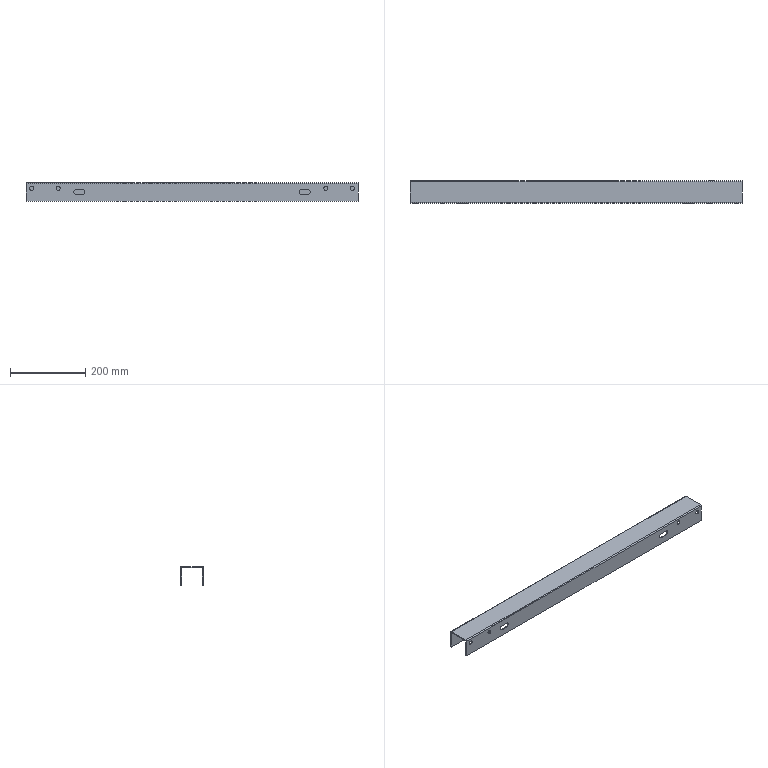Part | SolidWorks | features ICE 3, Cut 2, EdgeFlange 1, FlatPattern 1, SMBaseFlange 1, SheetMetal 1 | 1 solid | 44 faces | box 884 x 60 x 50 mm | volume 336431 mm3 | cylinder 22 | plane 22 | commonest cylinder face diameters 11 x8 10.5 x6 13 x4 0.4 x2 5.4 x2
STEP:
#1=CARTESIAN_POINT('',(-356.,-27.5,-20.5));
#2=VERTEX_POINT('',#1);
#3=CARTESIAN_POINT('',(-356.,-27.5,-9.5));
#4=VERTEX_POINT('',#3);
#5=CARTESIAN_POINT('',(-356.,-27.5,-15.));
#6=DIRECTION('',(0.,1.,0.));
#7=DIRECTION('',(0.,0.,1.));
#8=AXIS2_PLACEMENT_3D('',#5,#6,#7);
#9=CIRCLE('',#8,5.5);
#10=EDGE_CURVE('',#2,#4,#9,.T.);
#11=ORIENTED_EDGE('',*,*,#10,.T.);
#12=CARTESIAN_POINT('',(-356.,-30.,-9.5));
#13=VERTEX_POINT('',#12);
#14=CARTESIAN_POINT('',(-356.,-20.,-9.5));
#15=DIRECTION('',(0.,-1.,0.));
#16=VECTOR('',#15,1000.);
#17=LINE('',#14,#16);
#18=EDGE_CURVE('',#4,#13,#17,.T.);
#19=ORIENTED_EDGE('',*,*,#18,.T.);
#20=CARTESIAN_POINT('',(-356.,-30.,-20.5));
#21=VERTEX_POINT('',#20);
#22=CARTESIAN_POINT('',(-356.,-30.,-15.));
#23=DIRECTION('',(0.,-1.,0.));
#24=DIRECTION('',(0.,0.,1.));
#25=AXIS2_PLACEMENT_3D('',#22,#23,#24);
#26=CIRCLE('',#25,5.5);
#27=EDGE_CURVE('',#13,#21,#26,.T.);
#28=ORIENTED_EDGE('',*,*,#27,.T.);
#29=CARTESIAN_POINT('',(-356.,-20.,-20.5));
#30=DIRECTION('',(0.,-1.,0.));
#31=VECTOR('',#30,1000.);
#32=LINE('',#29,#31);
#33=EDGE_CURVE('',#2,#21,#32,.T.);
#34=ORIENTED_EDGE('',*,*,#33,.F.);
#35=EDGE_LOOP('',(#11,#19,#28,#34));
#36=FACE_OUTER_BOUND('',#35,.T.);
#37=CARTESIAN_POINT('',(-356.,-20.,-15.));
#38=DIRECTION('',(0.,-1.,0.));
#39=DIRECTION('',(0.,0.,-1.));
#40=AXIS2_PLACEMENT_3D('',#37,#38,#39);
#41=CYLINDRICAL_SURFACE('',#40,5.5);
#42=ADVANCED_FACE('',(#36),#41,.F.);
#43=CARTESIAN_POINT('',(-427.,-27.5,-20.5));
#44=VERTEX_POINT('',#43);
#45=CARTESIAN_POINT('',(-427.,-27.5,-9.5));
#46=VERTEX_POINT('',#45);
#47=CARTESIAN_POINT('',(-427.,-27.5,-15.));
#48=DIRECTION('',(0.,1.,0.));
#49=DIRECTION('',(0.,0.,1.));
#50=AXIS2_PLACEMENT_3D('',#47,#48,#49);
#51=CIRCLE('',#50,5.5);
#52=EDGE_CURVE('',#44,#46,#51,.T.);
#53=ORIENTED_EDGE('',*,*,#52,.T.);
#54=CARTESIAN_POINT('',(-427.,-30.,-9.5));
#55=VERTEX_POINT('',#54);
#56=CARTESIAN_POINT('',(-427.,-20.,-9.5));
#57=DIRECTION('',(0.,-1.,0.));
#58=VECTOR('',#57,1000.);
#59=LINE('',#56,#58);
#60=EDGE_CURVE('',#46,#55,#59,.T.);
#61=ORIENTED_EDGE('',*,*,#60,.T.);
#62=CARTESIAN_POINT('',(-427.,-30.,-20.5));
#63=VERTEX_POINT('',#62);
#64=CARTESIAN_POINT('',(-427.,-30.,-15.));
#65=DIRECTION('',(0.,-1.,0.));
#66=DIRECTION('',(0.,0.,1.));
#67=AXIS2_PLACEMENT_3D('',#64,#65,#66);
#68=CIRCLE('',#67,5.5);
#69=EDGE_CURVE('',#55,#63,#68,.T.);
#70=ORIENTED_EDGE('',*,*,#69,.T.);
#71=CARTESIAN_POINT('',(-427.,-20.,-20.5));
#72=DIRECTION('',(0.,-1.,0.));
#73=VECTOR('',#72,1000.);
#74=LINE('',#71,#73);
#75=EDGE_CURVE('',#44,#63,#74,.T.);
#76=ORIENTED_EDGE('',*,*,#75,.F.);
#77=EDGE_LOOP('',(#53,#61,#70,#76));
#78=FACE_OUTER_BOUND('',#77,.T.);
#79=CARTESIAN_POINT('',(-427.,-20.,-15.));
#80=DIRECTION('',(0.,-1.,0.));
#81=DIRECTION('',(0.,0.,-1.));
#82=AXIS2_PLACEMENT_3D('',#79,#80,#81);
#83=CYLINDRICAL_SURFACE('',#82,5.5);
#84=ADVANCED_FACE('',(#78),#83,.F.);
#85=CARTESIAN_POINT('',(427.,-27.5,-20.5));
#86=VERTEX_POINT('',#85);
#87=CARTESIAN_POINT('',(427.,-27.5,-9.5));
#88=VERTEX_POINT('',#87);
#89=CARTESIAN_POINT('',(427.,-27.5,-15.));
#90=DIRECTION('',(0.,1.,0.));
#91=DIRECTION('',(0.,0.,1.));
#92=AXIS2_PLACEMENT_3D('',#89,#90,#91);
#93=CIRCLE('',#92,5.5);
#94=EDGE_CURVE('',#86,#88,#93,.T.);
#95=ORIENTED_EDGE('',*,*,#94,.T.);
#96=CARTESIAN_POINT('',(427.,-30.,-9.5));
#97=VERTEX_POINT('',#96);
#98=CARTESIAN_POINT('',(427.,-20.,-9.5));
#99=DIRECTION('',(0.,-1.,0.));
#100=VECTOR('',#99,1000.);
#101=LINE('',#98,#100);
#102=EDGE_CURVE('',#88,#97,#101,.T.);
#103=ORIENTED_EDGE('',*,*,#102,.T.);
#104=CARTESIAN_POINT('',(427.,-30.,-20.5));
#105=VERTEX_POINT('',#104);
#106=CARTESIAN_POINT('',(427.,-30.,-15.));
#107=DIRECTION('',(0.,-1.,0.));
#108=DIRECTION('',(0.,0.,-1.));
#109=AXIS2_PLACEMENT_3D('',#106,#107,#108);
#110=CIRCLE('',#109,5.5);
#111=EDGE_CURVE('',#97,#105,#110,.T.);
#112=ORIENTED_EDGE('',*,*,#111,.T.);
#113=CARTESIAN_POINT('',(427.,-20.,-20.5));
#114=DIRECTION('',(0.,-1.,0.));
#115=VECTOR('',#114,1000.);
#116=LINE('',#113,#115);
#117=EDGE_CURVE('',#86,#105,#116,.T.);
#118=ORIENTED_EDGE('',*,*,#117,.F.);
#119=EDGE_LOOP('',(#95,#103,#112,#118));
#120=FACE_OUTER_BOUND('',#119,.T.);
#121=CARTESIAN_POINT('',(427.,-20.,-15.));
#122=DIRECTION('',(0.,-1.,0.));
#123=DIRECTION('',(0.,0.,-1.));
#124=AXIS2_PLACEMENT_3D('',#121,#122,#123);
#125=CYLINDRICAL_SURFACE('',#124,5.5);
#126=ADVANCED_FACE('',(#120),#125,.F.);
#127=CARTESIAN_POINT('',(356.,-27.5,-20.5));
#128=VERTEX_POINT('',#127);
#129=CARTESIAN_POINT('',(356.,-27.5,-9.5));
#130=VERTEX_POINT('',#129);
#131=CARTESIAN_POINT('',(356.,-27.5,-15.));
#132=DIRECTION('',(0.,1.,0.));
#133=DIRECTION('',(0.,0.,1.));
#134=AXIS2_PLACEMENT_3D('',#131,#132,#133);
#135=CIRCLE('',#134,5.5);
#136=EDGE_CURVE('',#128,#130,#135,.T.);
#137=ORIENTED_EDGE('',*,*,#136,.T.);
#138=CARTESIAN_POINT('',(356.,-30.,-9.5));
#139=VERTEX_POINT('',#138);
#140=CARTESIAN_POINT('',(356.,-20.,-9.5));
#141=DIRECTION('',(0.,-1.,0.));
#142=VECTOR('',#141,1000.);
#143=LINE('',#140,#142);
#144=EDGE_CURVE('',#130,#139,#143,.T.);
#145=ORIENTED_EDGE('',*,*,#144,.T.);
#146=CARTESIAN_POINT('',(356.,-30.,-20.5));
#147=VERTEX_POINT('',#146);
#148=CARTESIAN_POINT('',(356.,-30.,-15.));
#149=DIRECTION('',(0.,-1.,0.));
#150=DIRECTION('',(0.,0.,-1.));
#151=AXIS2_PLACEMENT_3D('',#148,#149,#150);
#152=CIRCLE('',#151,5.5);
#153=EDGE_CURVE('',#139,#147,#152,.T.);
#154=ORIENTED_EDGE('',*,*,#153,.T.);
#155=CARTESIAN_POINT('',(356.,-20.,-20.5));
#156=DIRECTION('',(0.,-1.,0.));
#157=VECTOR('',#156,1000.);
#158=LINE('',#155,#157);
#159=EDGE_CURVE('',#128,#147,#158,.T.);
#160=ORIENTED_EDGE('',*,*,#159,.F.);
#161=EDGE_LOOP('',(#137,#145,#154,#160));
#162=FACE_OUTER_BOUND('',#161,.T.);
#163=CARTESIAN_POINT('',(356.,-20.,-15.));
#164=DIRECTION('',(0.,-1.,0.));
#165=DIRECTION('',(0.,0.,-1.));
#166=AXIS2_PLACEMENT_3D('',#163,#164,#165);
#167=CYLINDRICAL_SURFACE('',#166,5.5);
#168=ADVANCED_FACE('',(#162),#167,.F.);
#169=CARTESIAN_POINT('',(360.,27.5,-30.25));
#170=VERTEX_POINT('',#169);
#171=CARTESIAN_POINT('',(360.,27.5,-19.75));
#172=VERTEX_POINT('',#171);
#173=CARTESIAN_POINT('',(360.,27.5,-25.));
#174=DIRECTION('',(0.,1.,0.));
#175=DIRECTION('',(0.,0.,1.));
#176=AXIS2_PLACEMENT_3D('',#173,#174,#175);
#177=CIRCLE('',#176,5.25);
#178=EDGE_CURVE('',#170,#172,#177,.T.);
#179=ORIENTED_EDGE('',*,*,#178,.F.);
#180=CARTESIAN_POINT('',(360.,30.,-30.25));
#181=VERTEX_POINT('',#180);
#182=CARTESIAN_POINT('',(360.,20.,-30.25));
#183=DIRECTION('',(0.,1.,0.));
#184=VECTOR('',#183,1000.);
#185=LINE('',#182,#184);
#186=EDGE_CURVE('',#170,#181,#185,.T.);
#187=ORIENTED_EDGE('',*,*,#186,.T.);
#188=CARTESIAN_POINT('',(360.,30.,-19.75));
#189=VERTEX_POINT('',#188);
#190=CARTESIAN_POINT('',(360.,30.,-25.));
#191=DIRECTION('',(0.,1.,0.));
#192=DIRECTION('',(0.,0.,1.));
#193=AXIS2_PLACEMENT_3D('',#190,#191,#192);
#194=CIRCLE('',#193,5.25);
#195=EDGE_CURVE('',#181,#189,#194,.T.);
#196=ORIENTED_EDGE('',*,*,#195,.T.);
#197=CARTESIAN_POINT('',(360.,20.,-19.75));
#198=DIRECTION('',(0.,1.,0.));
#199=VECTOR('',#198,1000.);
#200=LINE('',#197,#199);
#201=EDGE_CURVE('',#172,#189,#200,.T.);
#202=ORIENTED_EDGE('',*,*,#201,.F.);
#203=EDGE_LOOP('',(#179,#187,#196,#202));
#204=FACE_OUTER_BOUND('',#203,.T.);
#205=CARTESIAN_POINT('',(360.,20.,-25.));
#206=DIRECTION('',(0.,1.,0.));
#207=DIRECTION('',(0.,0.,1.));
#208=AXIS2_PLACEMENT_3D('',#205,#206,#207);
#209=CYLINDRICAL_SURFACE('',#208,5.25);
#210=ADVANCED_FACE('',(#204),#209,.F.);
#211=CARTESIAN_POINT('',(0.,27.5,-30.25));
#212=VERTEX_POINT('',#211);
#213=CARTESIAN_POINT('',(0.,27.5,-19.75));
#214=VERTEX_POINT('',#213);
#215=CARTESIAN_POINT('',(0.,27.5,-25.));
#216=DIRECTION('',(0.,1.,0.));
#217=DIRECTION('',(0.,0.,1.));
#218=AXIS2_PLACEMENT_3D('',#215,#216,#217);
#219=CIRCLE('',#218,5.25);
#220=EDGE_CURVE('',#212,#214,#219,.T.);
#221=ORIENTED_EDGE('',*,*,#220,.F.);
#222=CARTESIAN_POINT('',(0.,30.,-30.25));
#223=VERTEX_POINT('',#222);
#224=CARTESIAN_POINT('',(0.,20.,-30.25));
#225=DIRECTION('',(0.,1.,0.));
#226=VECTOR('',#225,1000.);
#227=LINE('',#224,#226);
#228=EDGE_CURVE('',#212,#223,#227,.T.);
#229=ORIENTED_EDGE('',*,*,#228,.T.);
#230=CARTESIAN_POINT('',(0.,30.,-19.75));
#231=VERTEX_POINT('',#230);
#232=CARTESIAN_POINT('',(0.,30.,-25.));
#233=DIRECTION('',(0.,1.,0.));
#234=DIRECTION('',(0.,0.,1.));
#235=AXIS2_PLACEMENT_3D('',#232,#233,#234);
#236=CIRCLE('',#235,5.25);
#237=EDGE_CURVE('',#223,#231,#236,.T.);
#238=ORIENTED_EDGE('',*,*,#237,.T.);
#239=CARTESIAN_POINT('',(0.,20.,-19.75));
#240=DIRECTION('',(0.,1.,0.));
#241=VECTOR('',#240,1000.);
#242=LINE('',#239,#241);
#243=EDGE_CURVE('',#214,#231,#242,.T.);
#244=ORIENTED_EDGE('',*,*,#243,.F.);
#245=EDGE_LOOP('',(#221,#229,#238,#244));
#246=FACE_OUTER_BOUND('',#245,.T.);
#247=CARTESIAN_POINT('',(0.,20.,-25.));
#248=DIRECTION('',(0.,1.,0.));
#249=DIRECTION('',(0.,0.,1.));
#250=AXIS2_PLACEMENT_3D('',#247,#248,#249);
#251=CYLINDRICAL_SURFACE('',#250,5.25);
#252=ADVANCED_FACE('',(#246),#251,.F.);
#253=CARTESIAN_POINT('',(-360.,27.5,-30.25));
#254=VERTEX_POINT('',#253);
#255=CARTESIAN_POINT('',(-360.,27.5,-19.75));
#256=VERTEX_POINT('',#255);
#257=CARTESIAN_POINT('',(-360.,27.5,-25.));
#258=DIRECTION('',(0.,1.,0.));
#259=DIRECTION('',(0.,0.,1.));
#260=AXIS2_PLACEMENT_3D('',#257,#258,#259);
#261=CIRCLE('',#260,5.25);
#262=EDGE_CURVE('',#254,#256,#261,.T.);
#263=ORIENTED_EDGE('',*,*,#262,.F.);
#264=CARTESIAN_POINT('',(-360.,30.,-30.25));
#265=VERTEX_POINT('',#264);
#266=CARTESIAN_POINT('',(-360.,20.,-30.25));
#267=DIRECTION('',(0.,1.,0.));
#268=VECTOR('',#267,1000.);
#269=LINE('',#266,#268);
#270=EDGE_CURVE('',#254,#265,#269,.T.);
#271=ORIENTED_EDGE('',*,*,#270,.T.);
#272=CARTESIAN_POINT('',(-360.,30.,-19.75));
#273=VERTEX_POINT('',#272);
#274=CARTESIAN_POINT('',(-360.,30.,-25.));
#275=DIRECTION('',(0.,1.,0.));
#276=DIRECTION('',(0.,0.,1.));
#277=AXIS2_PLACEMENT_3D('',#274,#275,#276);
#278=CIRCLE('',#277,5.25);
#279=EDGE_CURVE('',#265,#273,#278,.T.);
#280=ORIENTED_EDGE('',*,*,#279,.T.);
#281=CARTESIAN_POINT('',(-360.,20.,-19.75));
#282=DIRECTION('',(0.,1.,0.));
#283=VECTOR('',#282,1000.);
#284=LINE('',#281,#283);
#285=EDGE_CURVE('',#256,#273,#284,.T.);
#286=ORIENTED_EDGE('',*,*,#285,.F.);
#287=EDGE_LOOP('',(#263,#271,#280,#286));
#288=FACE_OUTER_BOUND('',#287,.T.);
#289=CARTESIAN_POINT('',(-360.,20.,-25.));
#290=DIRECTION('',(0.,1.,0.));
#291=DIRECTION('',(0.,0.,1.));
#292=AXIS2_PLACEMENT_3D('',#289,#290,#291);
#293=CYLINDRICAL_SURFACE('',#292,5.25);
#294=ADVANCED_FACE('',(#288),#293,.F.);
#295=CARTESIAN_POINT('',(-442.,-27.3,-2.5));
#296=VERTEX_POINT('',#295);
#297=CARTESIAN_POINT('',(442.,-27.3,-2.5));
#298=VERTEX_POINT('',#297);
#299=CARTESIAN_POINT('',(-442.,-27.3,-2.5));
#300=DIRECTION('',(1.,0.,0.));
#301=VECTOR('',#300,1000.);
#302=LINE('',#299,#301);
#303=EDGE_CURVE('',#296,#298,#302,.T.);
#304=ORIENTED_EDGE('',*,*,#303,.F.);
#305=CARTESIAN_POINT('',(-442.,27.3,-2.5));
#306=VERTEX_POINT('',#305);
#307=CARTESIAN_POINT('',(-442.,30.,-2.5));
#308=DIRECTION('',(0.,-1.,0.));
#309=VECTOR('',#308,1000.);
#310=LINE('',#307,#309);
#311=EDGE_CURVE('',#306,#296,#310,.T.);
#312=ORIENTED_EDGE('',*,*,#311,.F.);
#313=CARTESIAN_POINT('',(442.,27.3,-2.5));
#314=VERTEX_POINT('',#313);
#315=CARTESIAN_POINT('',(442.,27.3,-2.5));
#316=DIRECTION('',(-1.,0.,0.));
#317=VECTOR('',#316,1000.);
#318=LINE('',#315,#317);
#319=EDGE_CURVE('',#314,#306,#318,.T.);
#320=ORIENTED_EDGE('',*,*,#319,.F.);
#321=CARTESIAN_POINT('',(442.,30.,-2.5));
#322=DIRECTION('',(0.,1.,0.));
#323=VECTOR('',#322,1000.);
#324=LINE('',#321,#323);
#325=EDGE_CURVE('',#298,#314,#324,.T.);
#326=ORIENTED_EDGE('',*,*,#325,.F.);
#327=EDGE_LOOP('',(#304,#312,#320,#326));
#328=FACE_OUTER_BOUND('',#327,.T.);
#329=CARTESIAN_POINT('',(0.,0.,-2.5));
#330=DIRECTION('',(0.,0.,1.));
#331=DIRECTION('',(1.,0.,0.));
#332=AXIS2_PLACEMENT_3D('',#329,#330,#331);
#333=PLANE('',#332);
#334=ADVANCED_FACE('',(#328),#333,.F.);
#335=CARTESIAN_POINT('',(-442.,27.3,0.));
#336=VERTEX_POINT('',#335);
#337=CARTESIAN_POINT('',(-442.,-27.3,0.));
#338=VERTEX_POINT('',#337);
#339=CARTESIAN_POINT('',(-442.,30.,0.));
#340=DIRECTION('',(0.,-1.,0.));
#341=VECTOR('',#340,1000.);
#342=LINE('',#339,#341);
#343=EDGE_CURVE('',#336,#338,#342,.T.);
#344=ORIENTED_EDGE('',*,*,#343,.T.);
#345=CARTESIAN_POINT('',(442.,-27.3,0.));
#346=VERTEX_POINT('',#345);
#347=CARTESIAN_POINT('',(-442.,-27.3,0.));
#348=DIRECTION('',(1.,0.,0.));
#349=VECTOR('',#348,1000.);
#350=LINE('',#347,#349);
#351=EDGE_CURVE('',#338,#346,#350,.T.);
#352=ORIENTED_EDGE('',*,*,#351,.T.);
#353=CARTESIAN_POINT('',(442.,27.3,0.));
#354=VERTEX_POINT('',#353);
#355=CARTESIAN_POINT('',(442.,30.,0.));
#356=DIRECTION('',(0.,1.,0.));
#357=VECTOR('',#356,1000.);
#358=LINE('',#355,#357);
#359=EDGE_CURVE('',#346,#354,#358,.T.);
#360=ORIENTED_EDGE('',*,*,#359,.T.);
#361=CARTESIAN_POINT('',(442.,27.3,0.));
#362=DIRECTION('',(-1.,0.,0.));
#363=VECTOR('',#362,1000.);
#364=LINE('',#361,#363);
#365=EDGE_CURVE('',#354,#336,#364,.T.);
#366=ORIENTED_EDGE('',*,*,#365,.T.);
#367=EDGE_LOOP('',(#344,#352,#360,#366));
#368=FACE_OUTER_BOUND('',#367,.T.);
#369=CARTESIAN_POINT('',(0.,0.,0.));
#370=DIRECTION('',(0.,0.,1.));
#371=DIRECTION('',(1.,0.,0.));
#372=AXIS2_PLACEMENT_3D('',#369,#370,#371);
#373=PLANE('',#372);
#374=ADVANCED_FACE('',(#368),#373,.T.);
#375=ORIENTED_EDGE('',*,*,#311,.T.);
#376=CARTESIAN_POINT('',(-442.,-27.3,-2.5));
#377=DIRECTION('',(0.,0.,1.));
#378=VECTOR('',#377,1000.);
#379=LINE('',#376,#378);
#380=EDGE_CURVE('',#296,#338,#379,.T.);
#381=ORIENTED_EDGE('',*,*,#380,.T.);
#382=ORIENTED_EDGE('',*,*,#343,.F.);
#383=CARTESIAN_POINT('',(-442.,27.3,-2.5));
#384=DIRECTION('',(0.,0.,1.));
#385=VECTOR('',#384,1000.);
#386=LINE('',#383,#385);
#387=EDGE_CURVE('',#306,#336,#386,.T.);
#388=ORIENTED_EDGE('',*,*,#387,.F.);
#389=EDGE_LOOP('',(#375,#381,#382,#388));
#390=FACE_OUTER_BOUND('',#389,.T.);
#391=CARTESIAN_POINT('',(-442.,30.,-2.5));
#392=DIRECTION('',(-1.,0.,0.));
#393=DIRECTION('',(0.,0.,1.));
#394=AXIS2_PLACEMENT_3D('',#391,#392,#393);
#395=PLANE('',#394);
#396=ADVANCED_FACE('',(#390),#395,.T.);
#397=CARTESIAN_POINT('',(442.,-27.3,-2.5));
#398=DIRECTION('',(0.,0.,1.));
#399=VECTOR('',#398,1000.);
#400=LINE('',#397,#399);
#401=EDGE_CURVE('',#298,#346,#400,.T.);
#402=ORIENTED_EDGE('',*,*,#401,.F.);
#403=ORIENTED_EDGE('',*,*,#325,.T.);
#404=CARTESIAN_POINT('',(442.,27.3,-2.5));
#405=DIRECTION('',(0.,0.,1.));
#406=VECTOR('',#405,1000.);
#407=LINE('',#404,#406);
#408=EDGE_CURVE('',#314,#354,#407,.T.);
#409=ORIENTED_EDGE('',*,*,#408,.T.);
#410=ORIENTED_EDGE('',*,*,#359,.F.);
#411=EDGE_LOOP('',(#402,#403,#409,#410));
#412=FACE_OUTER_BOUND('',#411,.T.);
#413=CARTESIAN_POINT('',(442.,30.,-2.5));
#414=DIRECTION('',(1.,0.,0.));
#415=DIRECTION('',(0.,0.,-1.));
#416=AXIS2_PLACEMENT_3D('',#413,#414,#415);
#417=PLANE('',#416);
#418=ADVANCED_FACE('',(#412),#417,.T.);
#419=CARTESIAN_POINT('',(-442.,27.5,-2.7));
#420=VERTEX_POINT('',#419);
#421=CARTESIAN_POINT('',(-442.,30.,-2.7));
#422=VERTEX_POINT('',#421);
#423=CARTESIAN_POINT('',(-442.,30.,-2.7));
#424=DIRECTION('',(0.,1.,0.));
#425=VECTOR('',#424,1000.);
#426=LINE('',#423,#425);
#427=EDGE_CURVE('',#420,#422,#426,.T.);
#428=ORIENTED_EDGE('',*,*,#427,.F.);
#429=CARTESIAN_POINT('',(-442.,27.3,-2.7));
#430=DIRECTION('',(-1.,0.,0.));
#431=DIRECTION('',(0.,0.,-1.));
#432=AXIS2_PLACEMENT_3D('',#429,#430,#431);
#433=CIRCLE('',#432,0.2);
#434=EDGE_CURVE('',#306,#420,#433,.T.);
#435=ORIENTED_EDGE('',*,*,#434,.F.);
#436=ORIENTED_EDGE('',*,*,#387,.T.);
#437=CARTESIAN_POINT('',(-442.,27.3,-2.7));
#438=DIRECTION('',(-1.,0.,0.));
#439=DIRECTION('',(0.,0.,-1.));
#440=AXIS2_PLACEMENT_3D('',#437,#438,#439);
#441=CIRCLE('',#440,2.7);
#442=EDGE_CURVE('',#336,#422,#441,.T.);
#443=ORIENTED_EDGE('',*,*,#442,.T.);
#444=EDGE_LOOP('',(#428,#435,#436,#443));
#445=FACE_OUTER_BOUND('',#444,.T.);
#446=CARTESIAN_POINT('',(-442.,27.3,-2.7));
#447=DIRECTION('',(-1.,0.,0.));
#448=DIRECTION('',(0.,0.,1.));
#449=AXIS2_PLACEMENT_3D('',#446,#447,#448);
#450=PLANE('',#449);
#451=ADVANCED_FACE('',(#445),#450,.T.);
#452=CARTESIAN_POINT('',(442.,27.5,-2.7));
#453=VERTEX_POINT('',#452);
#454=CARTESIAN_POINT('',(442.,27.3,-2.7));
#455=DIRECTION('',(1.,0.,0.));
#456=DIRECTION('',(0.,0.,-1.));
#457=AXIS2_PLACEMENT_3D('',#454,#455,#456);
#458=CIRCLE('',#457,0.2);
#459=EDGE_CURVE('',#453,#314,#458,.T.);
#460=ORIENTED_EDGE('',*,*,#459,.F.);
#461=CARTESIAN_POINT('',(442.,30.,-2.7));
#462=VERTEX_POINT('',#461);
#463=CARTESIAN_POINT('',(442.,27.5,-2.7));
#464=DIRECTION('',(0.,1.,0.));
#465=VECTOR('',#464,1000.);
#466=LINE('',#463,#465);
#467=EDGE_CURVE('',#453,#462,#466,.T.);
#468=ORIENTED_EDGE('',*,*,#467,.T.);
#469=CARTESIAN_POINT('',(442.,27.3,-2.7));
#470=DIRECTION('',(1.,0.,0.));
#471=DIRECTION('',(0.,0.,-1.));
#472=AXIS2_PLACEMENT_3D('',#469,#470,#471);
#473=CIRCLE('',#472,2.7);
#474=EDGE_CURVE('',#462,#354,#473,.T.);
#475=ORIENTED_EDGE('',*,*,#474,.T.);
#476=ORIENTED_EDGE('',*,*,#408,.F.);
#477=EDGE_LOOP('',(#460,#468,#475,#476));
#478=FACE_OUTER_BOUND('',#477,.T.);
#479=CARTESIAN_POINT('',(442.,27.3,-2.7));
#480=DIRECTION('',(-1.,0.,0.));
#481=DIRECTION('',(0.,0.,1.));
#482=AXIS2_PLACEMENT_3D('',#479,#480,#481);
#483=PLANE('',#482);
#484=ADVANCED_FACE('',(#478),#483,.F.);
#485=ORIENTED_EDGE('',*,*,#365,.F.);
#486=ORIENTED_EDGE('',*,*,#474,.F.);
#487=CARTESIAN_POINT('',(0.,30.,-2.7));
#488=DIRECTION('',(1.,0.,0.));
#489=VECTOR('',#488,1000.);
#490=LINE('',#487,#489);
#491=EDGE_CURVE('',#422,#462,#490,.T.);
#492=ORIENTED_EDGE('',*,*,#491,.F.);
#493=ORIENTED_EDGE('',*,*,#442,.F.);
#494=EDGE_LOOP('',(#485,#486,#492,#493));
#495=FACE_OUTER_BOUND('',#494,.T.);
#496=CARTESIAN_POINT('',(442.,27.3,-2.7));
#497=DIRECTION('',(1.,0.,0.));
#498=DIRECTION('',(0.,1.,0.));
#499=AXIS2_PLACEMENT_3D('',#496,#497,#498);
#500=CYLINDRICAL_SURFACE('',#499,2.7);
#501=ADVANCED_FACE('',(#495),#500,.T.);
#502=ORIENTED_EDGE('',*,*,#319,.T.);
#503=ORIENTED_EDGE('',*,*,#434,.T.);
#504=CARTESIAN_POINT('',(-442.,27.5,-2.7));
#505=DIRECTION('',(1.,0.,0.));
#506=VECTOR('',#505,1000.);
#507=LINE('',#504,#506);
#508=EDGE_CURVE('',#420,#453,#507,.T.);
#509=ORIENTED_EDGE('',*,*,#508,.T.);
#510=ORIENTED_EDGE('',*,*,#459,.T.);
#511=EDGE_LOOP('',(#502,#503,#509,#510));
#512=FACE_OUTER_BOUND('',#511,.T.);
#513=CARTESIAN_POINT('',(442.,27.3,-2.7));
#514=DIRECTION('',(1.,0.,0.));
#515=DIRECTION('',(0.,1.,0.));
#516=AXIS2_PLACEMENT_3D('',#513,#514,#515);
#517=CYLINDRICAL_SURFACE('',#516,0.2);
#518=ADVANCED_FACE('',(#512),#517,.F.);
#519=CARTESIAN_POINT('',(442.,30.,-50.));
#520=VERTEX_POINT('',#519);
#521=CARTESIAN_POINT('',(442.,30.,-2.5));
#522=DIRECTION('',(0.,0.,1.));
#523=VECTOR('',#522,1000.);
#524=LINE('',#521,#523);
#525=EDGE_CURVE('',#520,#462,#524,.T.);
#526=ORIENTED_EDGE('',*,*,#525,.T.);
#527=ORIENTED_EDGE('',*,*,#467,.F.);
#528=CARTESIAN_POINT('',(442.,27.5,-50.));
#529=VERTEX_POINT('',#528);
#530=CARTESIAN_POINT('',(442.,27.5,0.));
#531=DIRECTION('',(0.,0.,1.));
#532=VECTOR('',#531,1000.);
#533=LINE('',#530,#532);
#534=EDGE_CURVE('',#529,#453,#533,.T.);
#535=ORIENTED_EDGE('',*,*,#534,.F.);
#536=CARTESIAN_POINT('',(442.,30.,-50.));
#537=DIRECTION('',(0.,-1.,0.));
#538=VECTOR('',#537,1000.);
#539=LINE('',#536,#538);
#540=EDGE_CURVE('',#520,#529,#539,.T.);
#541=ORIENTED_EDGE('',*,*,#540,.F.);
#542=EDGE_LOOP('',(#526,#527,#535,#541));
#543=FACE_OUTER_BOUND('',#542,.T.);
#544=CARTESIAN_POINT('',(442.,30.,-2.5));
#545=DIRECTION('',(1.,0.,0.));
#546=DIRECTION('',(0.,0.,-1.));
#547=AXIS2_PLACEMENT_3D('',#544,#545,#546);
#548=PLANE('',#547);
#549=ADVANCED_FACE('',(#543),#548,.T.);
#550=CARTESIAN_POINT('',(-442.,27.5,-50.));
#551=VERTEX_POINT('',#550);
#552=CARTESIAN_POINT('',(-442.,27.5,0.));
#553=DIRECTION('',(0.,0.,-1.));
#554=VECTOR('',#553,1000.);
#555=LINE('',#552,#554);
#556=EDGE_CURVE('',#420,#551,#555,.T.);
#557=ORIENTED_EDGE('',*,*,#556,.F.);
#558=ORIENTED_EDGE('',*,*,#427,.T.);
#559=CARTESIAN_POINT('',(-442.,30.,-50.));
#560=VERTEX_POINT('',#559);
#561=CARTESIAN_POINT('',(-442.,30.,-50.));
#562=DIRECTION('',(0.,0.,-1.));
#563=VECTOR('',#562,1000.);
#564=LINE('',#561,#563);
#565=EDGE_CURVE('',#422,#560,#564,.T.);
#566=ORIENTED_EDGE('',*,*,#565,.T.);
#567=CARTESIAN_POINT('',(-442.,30.,-50.));
#568=DIRECTION('',(0.,-1.,0.));
#569=VECTOR('',#568,1000.);
#570=LINE('',#567,#569);
#571=EDGE_CURVE('',#560,#551,#570,.T.);
#572=ORIENTED_EDGE('',*,*,#571,.T.);
#573=EDGE_LOOP('',(#557,#558,#566,#572));
#574=FACE_OUTER_BOUND('',#573,.T.);
#575=CARTESIAN_POINT('',(-442.,30.,-50.));
#576=DIRECTION('',(-1.,0.,0.));
#577=DIRECTION('',(0.,0.,1.));
#578=AXIS2_PLACEMENT_3D('',#575,#576,#577);
#579=PLANE('',#578);
#580=ADVANCED_FACE('',(#574),#579,.T.);
#581=CARTESIAN_POINT('',(360.,30.,-25.));
#582=DIRECTION('',(0.,1.,0.));
#583=DIRECTION('',(0.,0.,1.));
#584=AXIS2_PLACEMENT_3D('',#581,#582,#583);
#585=CIRCLE('',#584,5.25);
#586=EDGE_CURVE('',#189,#181,#585,.T.);
#587=ORIENTED_EDGE('',*,*,#586,.F.);
#588=ORIENTED_EDGE('',*,*,#195,.F.);
#589=EDGE_LOOP('',(#587,#588));
#590=FACE_BOUND('',#589,.T.);
#591=CARTESIAN_POINT('',(0.,30.,-25.));
#592=DIRECTION('',(0.,1.,0.));
#593=DIRECTION('',(0.,0.,1.));
#594=AXIS2_PLACEMENT_3D('',#591,#592,#593);
#595=CIRCLE('',#594,5.25);
#596=EDGE_CURVE('',#231,#223,#595,.T.);
#597=ORIENTED_EDGE('',*,*,#596,.F.);
#598=ORIENTED_EDGE('',*,*,#237,.F.);
#599=EDGE_LOOP('',(#597,#598));
#600=FACE_BOUND('',#599,.T.);
#601=CARTESIAN_POINT('',(-360.,30.,-25.));
#602=DIRECTION('',(0.,1.,0.));
#603=DIRECTION('',(0.,0.,1.));
#604=AXIS2_PLACEMENT_3D('',#601,#602,#603);
#605=CIRCLE('',#604,5.25);
#606=EDGE_CURVE('',#273,#265,#605,.T.);
#607=ORIENTED_EDGE('',*,*,#606,.F.);
#608=ORIENTED_EDGE('',*,*,#279,.F.);
#609=EDGE_LOOP('',(#607,#608));
#610=FACE_BOUND('',#609,.T.);
#611=ORIENTED_EDGE('',*,*,#565,.F.);
#612=ORIENTED_EDGE('',*,*,#491,.T.);
#613=ORIENTED_EDGE('',*,*,#525,.F.);
#614=CARTESIAN_POINT('',(442.,30.,-50.));
#615=DIRECTION('',(1.,0.,0.));
#616=VECTOR('',#615,1000.);
#617=LINE('',#614,#616);
#618=EDGE_CURVE('',#560,#520,#617,.T.);
#619=ORIENTED_EDGE('',*,*,#618,.F.);
#620=EDGE_LOOP('',(#611,#612,#613,#619));
#621=FACE_OUTER_BOUND('',#620,.T.);
#622=CARTESIAN_POINT('',(0.,30.,0.));
#623=DIRECTION('',(0.,1.,0.));
#624=DIRECTION('',(0.,0.,1.));
#625=AXIS2_PLACEMENT_3D('',#622,#623,#624);
#626=PLANE('',#625);
#627=ADVANCED_FACE('',(#590,#600,#610,#621),#626,.T.);
#628=CARTESIAN_POINT('',(360.,27.5,-25.));
#629=DIRECTION('',(0.,1.,0.));
#630=DIRECTION('',(0.,0.,1.));
#631=AXIS2_PLACEMENT_3D('',#628,#629,#630);
#632=CIRCLE('',#631,5.25);
#633=EDGE_CURVE('',#172,#170,#632,.T.);
#634=ORIENTED_EDGE('',*,*,#633,.T.);
#635=ORIENTED_EDGE('',*,*,#178,.T.);
#636=EDGE_LOOP('',(#634,#635));
#637=FACE_BOUND('',#636,.T.);
#638=CARTESIAN_POINT('',(0.,27.5,-25.));
#639=DIRECTION('',(0.,1.,0.));
#640=DIRECTION('',(0.,0.,1.));
#641=AXIS2_PLACEMENT_3D('',#638,#639,#640);
#642=CIRCLE('',#641,5.25);
#643=EDGE_CURVE('',#214,#212,#642,.T.);
#644=ORIENTED_EDGE('',*,*,#643,.T.);
#645=ORIENTED_EDGE('',*,*,#220,.T.);
#646=EDGE_LOOP('',(#644,#645));
#647=FACE_BOUND('',#646,.T.);
#648=CARTESIAN_POINT('',(-360.,27.5,-25.));
#649=DIRECTION('',(0.,1.,0.));
#650=DIRECTION('',(0.,0.,1.));
#651=AXIS2_PLACEMENT_3D('',#648,#649,#650);
#652=CIRCLE('',#651,5.25);
#653=EDGE_CURVE('',#256,#254,#652,.T.);
#654=ORIENTED_EDGE('',*,*,#653,.T.);
#655=ORIENTED_EDGE('',*,*,#262,.T.);
#656=EDGE_LOOP('',(#654,#655));
#657=FACE_BOUND('',#656,.T.);
#658=ORIENTED_EDGE('',*,*,#508,.F.);
#659=ORIENTED_EDGE('',*,*,#556,.T.);
#660=CARTESIAN_POINT('',(0.,27.5,-50.));
#661=DIRECTION('',(1.,0.,0.));
#662=VECTOR('',#661,1000.);
#663=LINE('',#660,#662);
#664=EDGE_CURVE('',#551,#529,#663,.T.);
#665=ORIENTED_EDGE('',*,*,#664,.T.);
#666=ORIENTED_EDGE('',*,*,#534,.T.);
#667=EDGE_LOOP('',(#658,#659,#665,#666));
#668=FACE_OUTER_BOUND('',#667,.T.);
#669=CARTESIAN_POINT('',(0.,27.5,0.));
#670=DIRECTION('',(0.,1.,0.));
#671=DIRECTION('',(0.,0.,1.));
#672=AXIS2_PLACEMENT_3D('',#669,#670,#671);
#673=PLANE('',#672);
#674=ADVANCED_FACE('',(#637,#647,#657,#668),#673,.F.);
#675=ORIENTED_EDGE('',*,*,#664,.F.);
#676=ORIENTED_EDGE('',*,*,#571,.F.);
#677=ORIENTED_EDGE('',*,*,#618,.T.);
#678=ORIENTED_EDGE('',*,*,#540,.T.);
#679=EDGE_LOOP('',(#675,#676,#677,#678));
#680=FACE_OUTER_BOUND('',#679,.T.);
#681=CARTESIAN_POINT('',(442.,30.,-50.));
#682=DIRECTION('',(0.,0.,-1.));
#683=DIRECTION('',(0.,1.,0.));
#684=AXIS2_PLACEMENT_3D('',#681,#682,#683);
#685=PLANE('',#684);
#686=ADVANCED_FACE('',(#680),#685,.T.);
#687=CARTESIAN_POINT('',(442.,-27.5,-2.7));
#688=VERTEX_POINT('',#687);
#689=CARTESIAN_POINT('',(442.,-30.,-2.7));
#690=VERTEX_POINT('',#689);
#691=CARTESIAN_POINT('',(442.,-30.,-2.7));
#692=DIRECTION('',(0.,-1.,0.));
#693=VECTOR('',#692,1000.);
#694=LINE('',#691,#693);
#695=EDGE_CURVE('',#688,#690,#694,.T.);
#696=ORIENTED_EDGE('',*,*,#695,.F.);
#697=CARTESIAN_POINT('',(442.,-27.3,-2.7));
#698=DIRECTION('',(1.,0.,0.));
#699=DIRECTION('',(0.,0.,1.));
#700=AXIS2_PLACEMENT_3D('',#697,#698,#699);
#701=CIRCLE('',#700,0.2);
#702=EDGE_CURVE('',#298,#688,#701,.T.);
#703=ORIENTED_EDGE('',*,*,#702,.F.);
#704=ORIENTED_EDGE('',*,*,#401,.T.);
#705=CARTESIAN_POINT('',(442.,-27.3,-2.7));
#706=DIRECTION('',(1.,0.,0.));
#707=DIRECTION('',(0.,0.,1.));
#708=AXIS2_PLACEMENT_3D('',#705,#706,#707);
#709=CIRCLE('',#708,2.7);
#710=EDGE_CURVE('',#346,#690,#709,.T.);
#711=ORIENTED_EDGE('',*,*,#710,.T.);
#712=EDGE_LOOP('',(#696,#703,#704,#711));
#713=FACE_OUTER_BOUND('',#712,.T.);
#714=CARTESIAN_POINT('',(442.,-27.3,-2.7));
#715=DIRECTION('',(1.,0.,0.));
#716=DIRECTION('',(0.,0.,-1.));
#717=AXIS2_PLACEMENT_3D('',#714,#715,#716);
#718=PLANE('',#717);
#719=ADVANCED_FACE('',(#713),#718,.T.);
#720=CARTESIAN_POINT('',(-442.,-27.5,-2.7));
#721=VERTEX_POINT('',#720);
#722=CARTESIAN_POINT('',(-442.,-27.3,-2.7));
#723=DIRECTION('',(-1.,0.,0.));
#724=DIRECTION('',(0.,0.,1.));
#725=AXIS2_PLACEMENT_3D('',#722,#723,#724);
#726=CIRCLE('',#725,0.2);
#727=EDGE_CURVE('',#721,#296,#726,.T.);
#728=ORIENTED_EDGE('',*,*,#727,.F.);
#729=CARTESIAN_POINT('',(-442.,-30.,-2.7));
#730=VERTEX_POINT('',#729);
#731=CARTESIAN_POINT('',(-442.,-27.5,-2.7));
#732=DIRECTION('',(0.,-1.,0.));
#733=VECTOR('',#732,1000.);
#734=LINE('',#731,#733);
#735=EDGE_CURVE('',#721,#730,#734,.T.);
#736=ORIENTED_EDGE('',*,*,#735,.T.);
#737=CARTESIAN_POINT('',(-442.,-27.3,-2.7));
#738=DIRECTION('',(-1.,0.,0.));
#739=DIRECTION('',(0.,0.,1.));
#740=AXIS2_PLACEMENT_3D('',#737,#738,#739);
#741=CIRCLE('',#740,2.7);
#742=EDGE_CURVE('',#730,#338,#741,.T.);
#743=ORIENTED_EDGE('',*,*,#742,.T.);
#744=ORIENTED_EDGE('',*,*,#380,.F.);
#745=EDGE_LOOP('',(#728,#736,#743,#744));
#746=FACE_OUTER_BOUND('',#745,.T.);
#747=CARTESIAN_POINT('',(-442.,-27.3,-2.7));
#748=DIRECTION('',(1.,0.,0.));
#749=DIRECTION('',(0.,0.,-1.));
#750=AXIS2_PLACEMENT_3D('',#747,#748,#749);
#751=PLANE('',#750);
#752=ADVANCED_FACE('',(#746),#751,.F.);
#753=ORIENTED_EDGE('',*,*,#351,.F.);
#754=ORIENTED_EDGE('',*,*,#742,.F.);
#755=CARTESIAN_POINT('',(442.,-30.,-2.7));
#756=DIRECTION('',(1.,0.,0.));
#757=VECTOR('',#756,1000.);
#758=LINE('',#755,#757);
#759=EDGE_CURVE('',#730,#690,#758,.T.);
#760=ORIENTED_EDGE('',*,*,#759,.T.);
#761=ORIENTED_EDGE('',*,*,#710,.F.);
#762=EDGE_LOOP('',(#753,#754,#760,#761));
#763=FACE_OUTER_BOUND('',#762,.T.);
#764=CARTESIAN_POINT('',(-442.,-27.3,-2.7));
#765=DIRECTION('',(-1.,0.,0.));
#766=DIRECTION('',(0.,-1.,0.));
#767=AXIS2_PLACEMENT_3D('',#764,#765,#766);
#768=CYLINDRICAL_SURFACE('',#767,2.7);
#769=ADVANCED_FACE('',(#763),#768,.T.);
#770=ORIENTED_EDGE('',*,*,#303,.T.);
#771=ORIENTED_EDGE('',*,*,#702,.T.);
#772=CARTESIAN_POINT('',(442.,-27.5,-2.7));
#773=DIRECTION('',(-1.,0.,0.));
#774=VECTOR('',#773,1000.);
#775=LINE('',#772,#774);
#776=EDGE_CURVE('',#688,#721,#775,.T.);
#777=ORIENTED_EDGE('',*,*,#776,.T.);
#778=ORIENTED_EDGE('',*,*,#727,.T.);
#779=EDGE_LOOP('',(#770,#771,#777,#778));
#780=FACE_OUTER_BOUND('',#779,.T.);
#781=CARTESIAN_POINT('',(-442.,-27.3,-2.7));
#782=DIRECTION('',(-1.,0.,0.));
#783=DIRECTION('',(0.,-1.,0.));
#784=AXIS2_PLACEMENT_3D('',#781,#782,#783);
#785=CYLINDRICAL_SURFACE('',#784,0.2);
#786=ADVANCED_FACE('',(#780),#785,.F.);
#787=CARTESIAN_POINT('',(442.,-27.5,-50.));
#788=VERTEX_POINT('',#787);
#789=CARTESIAN_POINT('',(442.,-27.5,0.));
#790=DIRECTION('',(0.,0.,-1.));
#791=VECTOR('',#790,1000.);
#792=LINE('',#789,#791);
#793=EDGE_CURVE('',#688,#788,#792,.T.);
#794=ORIENTED_EDGE('',*,*,#793,.F.);
#795=ORIENTED_EDGE('',*,*,#695,.T.);
#796=CARTESIAN_POINT('',(442.,-30.,-50.));
#797=VERTEX_POINT('',#796);
#798=CARTESIAN_POINT('',(442.,-30.,-2.5));
#799=DIRECTION('',(0.,0.,-1.));
#800=VECTOR('',#799,1000.);
#801=LINE('',#798,#800);
#802=EDGE_CURVE('',#690,#797,#801,.T.);
#803=ORIENTED_EDGE('',*,*,#802,.T.);
#804=CARTESIAN_POINT('',(442.,-30.,-50.));
#805=DIRECTION('',(0.,1.,0.));
#806=VECTOR('',#805,1000.);
#807=LINE('',#804,#806);
#808=EDGE_CURVE('',#797,#788,#807,.T.);
#809=ORIENTED_EDGE('',*,*,#808,.T.);
#810=EDGE_LOOP('',(#794,#795,#803,#809));
#811=FACE_OUTER_BOUND('',#810,.T.);
#812=CARTESIAN_POINT('',(442.,-30.,-2.5));
#813=DIRECTION('',(1.,0.,0.));
#814=DIRECTION('',(0.,0.,-1.));
#815=AXIS2_PLACEMENT_3D('',#812,#813,#814);
#816=PLANE('',#815);
#817=ADVANCED_FACE('',(#811),#816,.T.);
#818=CARTESIAN_POINT('',(-442.,-30.,-50.));
#819=VERTEX_POINT('',#818);
#820=CARTESIAN_POINT('',(-442.,-30.,-50.));
#821=DIRECTION('',(0.,0.,1.));
#822=VECTOR('',#821,1000.);
#823=LINE('',#820,#822);
#824=EDGE_CURVE('',#819,#730,#823,.T.);
#825=ORIENTED_EDGE('',*,*,#824,.T.);
#826=ORIENTED_EDGE('',*,*,#735,.F.);
#827=CARTESIAN_POINT('',(-442.,-27.5,-50.));
#828=VERTEX_POINT('',#827);
#829=CARTESIAN_POINT('',(-442.,-27.5,0.));
#830=DIRECTION('',(0.,0.,1.));
#831=VECTOR('',#830,1000.);
#832=LINE('',#829,#831);
#833=EDGE_CURVE('',#828,#721,#832,.T.);
#834=ORIENTED_EDGE('',*,*,#833,.F.);
#835=CARTESIAN_POINT('',(-442.,-30.,-50.));
#836=DIRECTION('',(0.,1.,0.));
#837=VECTOR('',#836,1000.);
#838=LINE('',#835,#837);
#839=EDGE_CURVE('',#819,#828,#838,.T.);
#840=ORIENTED_EDGE('',*,*,#839,.F.);
#841=EDGE_LOOP('',(#825,#826,#834,#840));
#842=FACE_OUTER_BOUND('',#841,.T.);
#843=CARTESIAN_POINT('',(-442.,-30.,-50.));
#844=DIRECTION('',(-1.,0.,0.));
#845=DIRECTION('',(0.,0.,1.));
#846=AXIS2_PLACEMENT_3D('',#843,#844,#845);
#847=PLANE('',#846);
#848=ADVANCED_FACE('',(#842),#847,.T.);
#849=CARTESIAN_POINT('',(-356.,-30.,-15.));
#850=DIRECTION('',(0.,-1.,0.));
#851=DIRECTION('',(0.,0.,1.));
#852=AXIS2_PLACEMENT_3D('',#849,#850,#851);
#853=CIRCLE('',#852,5.5);
#854=EDGE_CURVE('',#21,#13,#853,.T.);
#855=ORIENTED_EDGE('',*,*,#854,.F.);
#856=ORIENTED_EDGE('',*,*,#27,.F.);
#857=EDGE_LOOP('',(#855,#856));
#858=FACE_BOUND('',#857,.T.);
#859=CARTESIAN_POINT('',(-427.,-30.,-15.));
#860=DIRECTION('',(0.,-1.,0.));
#861=DIRECTION('',(0.,0.,1.));
#862=AXIS2_PLACEMENT_3D('',#859,#860,#861);
#863=CIRCLE('',#862,5.5);
#864=EDGE_CURVE('',#63,#55,#863,.T.);
#865=ORIENTED_EDGE('',*,*,#864,.F.);
#866=ORIENTED_EDGE('',*,*,#69,.F.);
#867=EDGE_LOOP('',(#865,#866));
#868=FACE_BOUND('',#867,.T.);
#869=CARTESIAN_POINT('',(427.,-30.,-15.));
#870=DIRECTION('',(0.,-1.,0.));
#871=DIRECTION('',(0.,0.,-1.));
#872=AXIS2_PLACEMENT_3D('',#869,#870,#871);
#873=CIRCLE('',#872,5.5);
#874=EDGE_CURVE('',#105,#97,#873,.T.);
#875=ORIENTED_EDGE('',*,*,#874,.F.);
#876=ORIENTED_EDGE('',*,*,#111,.F.);
#877=EDGE_LOOP('',(#875,#876));
#878=FACE_BOUND('',#877,.T.);
#879=CARTESIAN_POINT('',(356.,-30.,-15.));
#880=DIRECTION('',(0.,-1.,0.));
#881=DIRECTION('',(0.,0.,-1.));
#882=AXIS2_PLACEMENT_3D('',#879,#880,#881);
#883=CIRCLE('',#882,5.5);
#884=EDGE_CURVE('',#147,#139,#883,.T.);
#885=ORIENTED_EDGE('',*,*,#884,.F.);
#886=ORIENTED_EDGE('',*,*,#153,.F.);
#887=EDGE_LOOP('',(#885,#886));
#888=FACE_BOUND('',#887,.T.);
#889=CARTESIAN_POINT('',(308.5,-30.,-18.5));
#890=VERTEX_POINT('',#889);
#891=CARTESIAN_POINT('',(291.5,-30.,-18.5));
#892=VERTEX_POINT('',#891);
#893=CARTESIAN_POINT('',(308.5,-30.,-18.5));
#894=DIRECTION('',(-1.,0.,0.));
#895=VECTOR('',#894,1000.);
#896=LINE('',#893,#895);
#897=EDGE_CURVE('',#890,#892,#896,.T.);
#898=ORIENTED_EDGE('',*,*,#897,.F.);
#899=CARTESIAN_POINT('',(308.5,-30.,-31.5));
#900=VERTEX_POINT('',#899);
#901=CARTESIAN_POINT('',(308.5,-30.,-25.));
#902=DIRECTION('',(0.,-1.,0.));
#903=DIRECTION('',(0.,0.,1.));
#904=AXIS2_PLACEMENT_3D('',#901,#902,#903);
#905=CIRCLE('',#904,6.5);
#906=EDGE_CURVE('',#900,#890,#905,.T.);
#907=ORIENTED_EDGE('',*,*,#906,.F.);
#908=CARTESIAN_POINT('',(291.5,-30.,-31.5));
#909=VERTEX_POINT('',#908);
#910=CARTESIAN_POINT('',(308.5,-30.,-31.5));
#911=DIRECTION('',(1.,0.,0.));
#912=VECTOR('',#911,1000.);
#913=LINE('',#910,#912);
#914=EDGE_CURVE('',#909,#900,#913,.T.);
#915=ORIENTED_EDGE('',*,*,#914,.F.);
#916=CARTESIAN_POINT('',(291.5,-30.,-25.));
#917=DIRECTION('',(0.,-1.,0.));
#918=DIRECTION('',(0.,0.,1.));
#919=AXIS2_PLACEMENT_3D('',#916,#917,#918);
#920=CIRCLE('',#919,6.5);
#921=EDGE_CURVE('',#892,#909,#920,.T.);
#922=ORIENTED_EDGE('',*,*,#921,.F.);
#923=EDGE_LOOP('',(#898,#907,#915,#922));
#924=FACE_BOUND('',#923,.T.);
#925=CARTESIAN_POINT('',(-308.5,-30.,-31.5));
#926=VERTEX_POINT('',#925);
#927=CARTESIAN_POINT('',(-291.5,-30.,-31.5));
#928=VERTEX_POINT('',#927);
#929=CARTESIAN_POINT('',(-308.5,-30.,-31.5));
#930=DIRECTION('',(1.,0.,0.));
#931=VECTOR('',#930,1000.);
#932=LINE('',#929,#931);
#933=EDGE_CURVE('',#926,#928,#932,.T.);
#934=ORIENTED_EDGE('',*,*,#933,.F.);
#935=CARTESIAN_POINT('',(-308.5,-30.,-18.5));
#936=VERTEX_POINT('',#935);
#937=CARTESIAN_POINT('',(-308.5,-30.,-25.));
#938=DIRECTION('',(0.,-1.,0.));
#939=DIRECTION('',(0.,0.,-1.));
#940=AXIS2_PLACEMENT_3D('',#937,#938,#939);
#941=CIRCLE('',#940,6.5);
#942=EDGE_CURVE('',#936,#926,#941,.T.);
#943=ORIENTED_EDGE('',*,*,#942,.F.);
#944=CARTESIAN_POINT('',(-291.5,-30.,-18.5));
#945=VERTEX_POINT('',#944);
#946=CARTESIAN_POINT('',(-308.5,-30.,-18.5));
#947=DIRECTION('',(-1.,0.,0.));
#948=VECTOR('',#947,1000.);
#949=LINE('',#946,#948);
#950=EDGE_CURVE('',#945,#936,#949,.T.);
#951=ORIENTED_EDGE('',*,*,#950,.F.);
#952=CARTESIAN_POINT('',(-291.5,-30.,-25.));
#953=DIRECTION('',(0.,-1.,0.));
#954=DIRECTION('',(0.,0.,-1.));
#955=AXIS2_PLACEMENT_3D('',#952,#953,#954);
#956=CIRCLE('',#955,6.5);
#957=EDGE_CURVE('',#928,#945,#956,.T.);
#958=ORIENTED_EDGE('',*,*,#957,.F.);
#959=EDGE_LOOP('',(#934,#943,#951,#958));
#960=FACE_BOUND('',#959,.T.);
#961=ORIENTED_EDGE('',*,*,#759,.F.);
#962=ORIENTED_EDGE('',*,*,#824,.F.);
#963=CARTESIAN_POINT('',(442.,-30.,-50.));
#964=DIRECTION('',(-1.,0.,0.));
#965=VECTOR('',#964,1000.);
#966=LINE('',#963,#965);
#967=EDGE_CURVE('',#797,#819,#966,.T.);
#968=ORIENTED_EDGE('',*,*,#967,.F.);
#969=ORIENTED_EDGE('',*,*,#802,.F.);
#970=EDGE_LOOP('',(#961,#962,#968,#969));
#971=FACE_OUTER_BOUND('',#970,.T.);
#972=CARTESIAN_POINT('',(0.,-30.,0.));
#973=DIRECTION('',(0.,1.,0.));
#974=DIRECTION('',(0.,0.,1.));
#975=AXIS2_PLACEMENT_3D('',#972,#973,#974);
#976=PLANE('',#975);
#977=ADVANCED_FACE('',(#858,#868,#878,#888,#924,#960,#971),#976,.F.);
#978=ORIENTED_EDGE('',*,*,#10,.F.);
#979=CARTESIAN_POINT('',(-356.,-27.5,-15.));
#980=DIRECTION('',(0.,1.,0.));
#981=DIRECTION('',(0.,0.,1.));
#982=AXIS2_PLACEMENT_3D('',#979,#980,#981);
#983=CIRCLE('',#982,5.5);
#984=EDGE_CURVE('',#4,#2,#983,.T.);
#985=ORIENTED_EDGE('',*,*,#984,.F.);
#986=EDGE_LOOP('',(#978,#985));
#987=FACE_BOUND('',#986,.T.);
#988=ORIENTED_EDGE('',*,*,#52,.F.);
#989=CARTESIAN_POINT('',(-427.,-27.5,-15.));
#990=DIRECTION('',(0.,1.,0.));
#991=DIRECTION('',(0.,0.,1.));
#992=AXIS2_PLACEMENT_3D('',#989,#990,#991);
#993=CIRCLE('',#992,5.5);
#994=EDGE_CURVE('',#46,#44,#993,.T.);
#995=ORIENTED_EDGE('',*,*,#994,.F.);
#996=EDGE_LOOP('',(#988,#995));
#997=FACE_BOUND('',#996,.T.);
#998=ORIENTED_EDGE('',*,*,#94,.F.);
#999=CARTESIAN_POINT('',(427.,-27.5,-15.));
#1000=DIRECTION('',(0.,1.,0.));
#1001=DIRECTION('',(0.,0.,1.));
#1002=AXIS2_PLACEMENT_3D('',#999,#1000,#1001);
#1003=CIRCLE('',#1002,5.5);
#1004=EDGE_CURVE('',#88,#86,#1003,.T.);
#1005=ORIENTED_EDGE('',*,*,#1004,.F.);
#1006=EDGE_LOOP('',(#998,#1005));
#1007=FACE_BOUND('',#1006,.T.);
#1008=ORIENTED_EDGE('',*,*,#136,.F.);
#1009=CARTESIAN_POINT('',(356.,-27.5,-15.));
#1010=DIRECTION('',(0.,1.,0.));
#1011=DIRECTION('',(0.,0.,1.));
#1012=AXIS2_PLACEMENT_3D('',#1009,#1010,#1011);
#1013=CIRCLE('',#1012,5.5);
#1014=EDGE_CURVE('',#130,#128,#1013,.T.);
#1015=ORIENTED_EDGE('',*,*,#1014,.F.);
#1016=EDGE_LOOP('',(#1008,#1015));
#1017=FACE_BOUND('',#1016,.T.);
#1018=CARTESIAN_POINT('',(308.5,-27.5,-18.5));
#1019=VERTEX_POINT('',#1018);
#1020=CARTESIAN_POINT('',(308.5,-27.5,-31.5));
#1021=VERTEX_POINT('',#1020);
#1022=CARTESIAN_POINT('',(308.5,-27.5,-25.));
#1023=DIRECTION('',(0.,1.,0.));
#1024=DIRECTION('',(0.,0.,1.));
#1025=AXIS2_PLACEMENT_3D('',#1022,#1023,#1024);
#1026=CIRCLE('',#1025,6.5);
#1027=EDGE_CURVE('',#1019,#1021,#1026,.T.);
#1028=ORIENTED_EDGE('',*,*,#1027,.F.);
#1029=CARTESIAN_POINT('',(291.5,-27.5,-18.5));
#1030=VERTEX_POINT('',#1029);
#1031=CARTESIAN_POINT('',(0.,-27.5,-18.5));
#1032=DIRECTION('',(1.,0.,0.));
#1033=VECTOR('',#1032,1000.);
#1034=LINE('',#1031,#1033);
#1035=EDGE_CURVE('',#1030,#1019,#1034,.T.);
#1036=ORIENTED_EDGE('',*,*,#1035,.F.);
#1037=CARTESIAN_POINT('',(291.5,-27.5,-31.5));
#1038=VERTEX_POINT('',#1037);
#1039=CARTESIAN_POINT('',(291.5,-27.5,-25.));
#1040=DIRECTION('',(0.,1.,0.));
#1041=DIRECTION('',(0.,0.,1.));
#1042=AXIS2_PLACEMENT_3D('',#1039,#1040,#1041);
#1043=CIRCLE('',#1042,6.5);
#1044=EDGE_CURVE('',#1038,#1030,#1043,.T.);
#1045=ORIENTED_EDGE('',*,*,#1044,.F.);
#1046=CARTESIAN_POINT('',(0.,-27.5,-31.5));
#1047=DIRECTION('',(-1.,0.,0.));
#1048=VECTOR('',#1047,1000.);
#1049=LINE('',#1046,#1048);
#1050=EDGE_CURVE('',#1021,#1038,#1049,.T.);
#1051=ORIENTED_EDGE('',*,*,#1050,.F.);
#1052=EDGE_LOOP('',(#1028,#1036,#1045,#1051));
#1053=FACE_BOUND('',#1052,.T.);
#1054=CARTESIAN_POINT('',(-308.5,-27.5,-31.5));
#1055=VERTEX_POINT('',#1054);
#1056=CARTESIAN_POINT('',(-308.5,-27.5,-18.5));
#1057=VERTEX_POINT('',#1056);
#1058=CARTESIAN_POINT('',(-308.5,-27.5,-25.));
#1059=DIRECTION('',(0.,1.,0.));
#1060=DIRECTION('',(0.,0.,1.));
#1061=AXIS2_PLACEMENT_3D('',#1058,#1059,#1060);
#1062=CIRCLE('',#1061,6.5);
#1063=EDGE_CURVE('',#1055,#1057,#1062,.T.);
#1064=ORIENTED_EDGE('',*,*,#1063,.F.);
#1065=CARTESIAN_POINT('',(-291.5,-27.5,-31.5));
#1066=VERTEX_POINT('',#1065);
#1067=CARTESIAN_POINT('',(0.,-27.5,-31.5));
#1068=DIRECTION('',(-1.,0.,0.));
#1069=VECTOR('',#1068,1000.);
#1070=LINE('',#1067,#1069);
#1071=EDGE_CURVE('',#1066,#1055,#1070,.T.);
#1072=ORIENTED_EDGE('',*,*,#1071,.F.);
#1073=CARTESIAN_POINT('',(-291.5,-27.5,-18.5));
#1074=VERTEX_POINT('',#1073);
#1075=CARTESIAN_POINT('',(-291.5,-27.5,-25.));
#1076=DIRECTION('',(0.,1.,0.));
#1077=DIRECTION('',(0.,0.,1.));
#1078=AXIS2_PLACEMENT_3D('',#1075,#1076,#1077);
#1079=CIRCLE('',#1078,6.5);
#1080=EDGE_CURVE('',#1074,#1066,#1079,.T.);
#1081=ORIENTED_EDGE('',*,*,#1080,.F.);
#1082=CARTESIAN_POINT('',(0.,-27.5,-18.5));
#1083=DIRECTION('',(1.,0.,0.));
#1084=VECTOR('',#1083,1000.);
#1085=LINE('',#1082,#1084);
#1086=EDGE_CURVE('',#1057,#1074,#1085,.T.);
#1087=ORIENTED_EDGE('',*,*,#1086,.F.);
#1088=EDGE_LOOP('',(#1064,#1072,#1081,#1087));
#1089=FACE_BOUND('',#1088,.T.);
#1090=ORIENTED_EDGE('',*,*,#833,.T.);
#1091=ORIENTED_EDGE('',*,*,#776,.F.);
#1092=ORIENTED_EDGE('',*,*,#793,.T.);
#1093=CARTESIAN_POINT('',(0.,-27.5,-50.));
#1094=DIRECTION('',(-1.,0.,0.));
#1095=VECTOR('',#1094,1000.);
#1096=LINE('',#1093,#1095);
#1097=EDGE_CURVE('',#788,#828,#1096,.T.);
#1098=ORIENTED_EDGE('',*,*,#1097,.T.);
#1099=EDGE_LOOP('',(#1090,#1091,#1092,#1098));
#1100=FACE_OUTER_BOUND('',#1099,.T.);
#1101=CARTESIAN_POINT('',(0.,-27.5,0.));
#1102=DIRECTION('',(0.,1.,0.));
#1103=DIRECTION('',(0.,0.,1.));
#1104=AXIS2_PLACEMENT_3D('',#1101,#1102,#1103);
#1105=PLANE('',#1104);
#1106=ADVANCED_FACE('',(#987,#997,#1007,#1017,#1053,#1089,#1100),#1105,.T.);
#1107=ORIENTED_EDGE('',*,*,#1097,.F.);
#1108=ORIENTED_EDGE('',*,*,#808,.F.);
#1109=ORIENTED_EDGE('',*,*,#967,.T.);
#1110=ORIENTED_EDGE('',*,*,#839,.T.);
#1111=EDGE_LOOP('',(#1107,#1108,#1109,#1110));
#1112=FACE_OUTER_BOUND('',#1111,.T.);
#1113=CARTESIAN_POINT('',(442.,-30.,-50.));
#1114=DIRECTION('',(0.,0.,-1.));
#1115=DIRECTION('',(0.,1.,0.));
#1116=AXIS2_PLACEMENT_3D('',#1113,#1114,#1115);
#1117=PLANE('',#1116);
#1118=ADVANCED_FACE('',(#1112),#1117,.T.);
#1119=ORIENTED_EDGE('',*,*,#270,.F.);
#1120=ORIENTED_EDGE('',*,*,#653,.F.);
#1121=ORIENTED_EDGE('',*,*,#285,.T.);
#1122=ORIENTED_EDGE('',*,*,#606,.T.);
#1123=EDGE_LOOP('',(#1119,#1120,#1121,#1122));
#1124=FACE_OUTER_BOUND('',#1123,.T.);
#1125=CARTESIAN_POINT('',(-360.,20.,-25.));
#1126=DIRECTION('',(0.,1.,0.));
#1127=DIRECTION('',(0.,0.,1.));
#1128=AXIS2_PLACEMENT_3D('',#1125,#1126,#1127);
#1129=CYLINDRICAL_SURFACE('',#1128,5.25);
#1130=ADVANCED_FACE('',(#1124),#1129,.F.);
#1131=ORIENTED_EDGE('',*,*,#228,.F.);
#1132=ORIENTED_EDGE('',*,*,#643,.F.);
#1133=ORIENTED_EDGE('',*,*,#243,.T.);
#1134=ORIENTED_EDGE('',*,*,#596,.T.);
#1135=EDGE_LOOP('',(#1131,#1132,#1133,#1134));
#1136=FACE_OUTER_BOUND('',#1135,.T.);
#1137=CARTESIAN_POINT('',(0.,20.,-25.));
#1138=DIRECTION('',(0.,1.,0.));
#1139=DIRECTION('',(0.,0.,1.));
#1140=AXIS2_PLACEMENT_3D('',#1137,#1138,#1139);
#1141=CYLINDRICAL_SURFACE('',#1140,5.25);
#1142=ADVANCED_FACE('',(#1136),#1141,.F.);
#1143=ORIENTED_EDGE('',*,*,#186,.F.);
#1144=ORIENTED_EDGE('',*,*,#633,.F.);
#1145=ORIENTED_EDGE('',*,*,#201,.T.);
#1146=ORIENTED_EDGE('',*,*,#586,.T.);
#1147=EDGE_LOOP('',(#1143,#1144,#1145,#1146));
#1148=FACE_OUTER_BOUND('',#1147,.T.);
#1149=CARTESIAN_POINT('',(360.,20.,-25.));
#1150=DIRECTION('',(0.,1.,0.));
#1151=DIRECTION('',(0.,0.,1.));
#1152=AXIS2_PLACEMENT_3D('',#1149,#1150,#1151);
#1153=CYLINDRICAL_SURFACE('',#1152,5.25);
#1154=ADVANCED_FACE('',(#1148),#1153,.F.);
#1155=ORIENTED_EDGE('',*,*,#1063,.T.);
#1156=CARTESIAN_POINT('',(-308.5,-20.,-18.5));
#1157=DIRECTION('',(0.,-1.,0.));
#1158=VECTOR('',#1157,1000.);
#1159=LINE('',#1156,#1158);
#1160=EDGE_CURVE('',#1057,#936,#1159,.T.);
#1161=ORIENTED_EDGE('',*,*,#1160,.T.);
#1162=ORIENTED_EDGE('',*,*,#942,.T.);
#1163=CARTESIAN_POINT('',(-308.5,-20.,-31.5));
#1164=DIRECTION('',(0.,-1.,0.));
#1165=VECTOR('',#1164,1000.);
#1166=LINE('',#1163,#1165);
#1167=EDGE_CURVE('',#1055,#926,#1166,.T.);
#1168=ORIENTED_EDGE('',*,*,#1167,.F.);
#1169=EDGE_LOOP('',(#1155,#1161,#1162,#1168));
#1170=FACE_OUTER_BOUND('',#1169,.T.);
#1171=CARTESIAN_POINT('',(-308.5,-20.,-25.));
#1172=DIRECTION('',(0.,-1.,0.));
#1173=DIRECTION('',(0.,0.,-1.));
#1174=AXIS2_PLACEMENT_3D('',#1171,#1172,#1173);
#1175=CYLINDRICAL_SURFACE('',#1174,6.5);
#1176=ADVANCED_FACE('',(#1170),#1175,.F.);
#1177=ORIENTED_EDGE('',*,*,#1086,.T.);
#1178=CARTESIAN_POINT('',(-291.5,-20.,-18.5));
#1179=DIRECTION('',(0.,-1.,0.));
#1180=VECTOR('',#1179,1000.);
#1181=LINE('',#1178,#1180);
#1182=EDGE_CURVE('',#1074,#945,#1181,.T.);
#1183=ORIENTED_EDGE('',*,*,#1182,.T.);
#1184=ORIENTED_EDGE('',*,*,#950,.T.);
#1185=ORIENTED_EDGE('',*,*,#1160,.F.);
#1186=EDGE_LOOP('',(#1177,#1183,#1184,#1185));
#1187=FACE_OUTER_BOUND('',#1186,.T.);
#1188=CARTESIAN_POINT('',(-308.5,-20.,-18.5));
#1189=DIRECTION('',(0.,0.,1.));
#1190=DIRECTION('',(0.,-1.,0.));
#1191=AXIS2_PLACEMENT_3D('',#1188,#1189,#1190);
#1192=PLANE('',#1191);
#1193=ADVANCED_FACE('',(#1187),#1192,.F.);
#1194=ORIENTED_EDGE('',*,*,#1080,.T.);
#1195=CARTESIAN_POINT('',(-291.5,-20.,-31.5));
#1196=DIRECTION('',(0.,-1.,0.));
#1197=VECTOR('',#1196,1000.);
#1198=LINE('',#1195,#1197);
#1199=EDGE_CURVE('',#1066,#928,#1198,.T.);
#1200=ORIENTED_EDGE('',*,*,#1199,.T.);
#1201=ORIENTED_EDGE('',*,*,#957,.T.);
#1202=ORIENTED_EDGE('',*,*,#1182,.F.);
#1203=EDGE_LOOP('',(#1194,#1200,#1201,#1202));
#1204=FACE_OUTER_BOUND('',#1203,.T.);
#1205=CARTESIAN_POINT('',(-291.5,-20.,-25.));
#1206=DIRECTION('',(0.,-1.,0.));
#1207=DIRECTION('',(0.,0.,-1.));
#1208=AXIS2_PLACEMENT_3D('',#1205,#1206,#1207);
#1209=CYLINDRICAL_SURFACE('',#1208,6.5);
#1210=ADVANCED_FACE('',(#1204),#1209,.F.);
#1211=ORIENTED_EDGE('',*,*,#1071,.T.);
#1212=ORIENTED_EDGE('',*,*,#1167,.T.);
#1213=ORIENTED_EDGE('',*,*,#933,.T.);
#1214=ORIENTED_EDGE('',*,*,#1199,.F.);
#1215=EDGE_LOOP('',(#1211,#1212,#1213,#1214));
#1216=FACE_OUTER_BOUND('',#1215,.T.);
#1217=CARTESIAN_POINT('',(-308.5,-20.,-31.5));
#1218=DIRECTION('',(0.,0.,-1.));
#1219=DIRECTION('',(0.,1.,0.));
#1220=AXIS2_PLACEMENT_3D('',#1217,#1218,#1219);
#1221=PLANE('',#1220);
#1222=ADVANCED_FACE('',(#1216),#1221,.F.);
#1223=ORIENTED_EDGE('',*,*,#1027,.T.);
#1224=CARTESIAN_POINT('',(308.5,-20.,-31.5));
#1225=DIRECTION('',(0.,-1.,0.));
#1226=VECTOR('',#1225,1000.);
#1227=LINE('',#1224,#1226);
#1228=EDGE_CURVE('',#1021,#900,#1227,.T.);
#1229=ORIENTED_EDGE('',*,*,#1228,.T.);
#1230=ORIENTED_EDGE('',*,*,#906,.T.);
#1231=CARTESIAN_POINT('',(308.5,-20.,-18.5));
#1232=DIRECTION('',(0.,-1.,0.));
#1233=VECTOR('',#1232,1000.);
#1234=LINE('',#1231,#1233);
#1235=EDGE_CURVE('',#1019,#890,#1234,.T.);
#1236=ORIENTED_EDGE('',*,*,#1235,.F.);
#1237=EDGE_LOOP('',(#1223,#1229,#1230,#1236));
#1238=FACE_OUTER_BOUND('',#1237,.T.);
#1239=CARTESIAN_POINT('',(308.5,-20.,-25.));
#1240=DIRECTION('',(0.,-1.,0.));
#1241=DIRECTION('',(0.,0.,-1.));
#1242=AXIS2_PLACEMENT_3D('',#1239,#1240,#1241);
#1243=CYLINDRICAL_SURFACE('',#1242,6.5);
#1244=ADVANCED_FACE('',(#1238),#1243,.F.);
#1245=ORIENTED_EDGE('',*,*,#1050,.T.);
#1246=CARTESIAN_POINT('',(291.5,-20.,-31.5));
#1247=DIRECTION('',(0.,-1.,0.));
#1248=VECTOR('',#1247,1000.);
#1249=LINE('',#1246,#1248);
#1250=EDGE_CURVE('',#1038,#909,#1249,.T.);
#1251=ORIENTED_EDGE('',*,*,#1250,.T.);
#1252=ORIENTED_EDGE('',*,*,#914,.T.);
#1253=ORIENTED_EDGE('',*,*,#1228,.F.);
#1254=EDGE_LOOP('',(#1245,#1251,#1252,#1253));
#1255=FACE_OUTER_BOUND('',#1254,.T.);
#1256=CARTESIAN_POINT('',(308.5,-20.,-31.5));
#1257=DIRECTION('',(0.,0.,-1.));
#1258=DIRECTION('',(0.,1.,0.));
#1259=AXIS2_PLACEMENT_3D('',#1256,#1257,#1258);
#1260=PLANE('',#1259);
#1261=ADVANCED_FACE('',(#1255),#1260,.F.);
#1262=ORIENTED_EDGE('',*,*,#1044,.T.);
#1263=CARTESIAN_POINT('',(291.5,-20.,-18.5));
#1264=DIRECTION('',(0.,-1.,0.));
#1265=VECTOR('',#1264,1000.);
#1266=LINE('',#1263,#1265);
#1267=EDGE_CURVE('',#1030,#892,#1266,.T.);
#1268=ORIENTED_EDGE('',*,*,#1267,.T.);
#1269=ORIENTED_EDGE('',*,*,#921,.T.);
#1270=ORIENTED_EDGE('',*,*,#1250,.F.);
#1271=EDGE_LOOP('',(#1262,#1268,#1269,#1270));
#1272=FACE_OUTER_BOUND('',#1271,.T.);
#1273=CARTESIAN_POINT('',(291.5,-20.,-25.));
#1274=DIRECTION('',(0.,-1.,0.));
#1275=DIRECTION('',(0.,0.,-1.));
#1276=AXIS2_PLACEMENT_3D('',#1273,#1274,#1275);
#1277=CYLINDRICAL_SURFACE('',#1276,6.5);
#1278=ADVANCED_FACE('',(#1272),#1277,.F.);
#1279=ORIENTED_EDGE('',*,*,#1035,.T.);
#1280=ORIENTED_EDGE('',*,*,#1235,.T.);
#1281=ORIENTED_EDGE('',*,*,#897,.T.);
#1282=ORIENTED_EDGE('',*,*,#1267,.F.);
#1283=EDGE_LOOP('',(#1279,#1280,#1281,#1282));
#1284=FACE_OUTER_BOUND('',#1283,.T.);
#1285=CARTESIAN_POINT('',(308.5,-20.,-18.5));
#1286=DIRECTION('',(0.,0.,1.));
#1287=DIRECTION('',(1.,0.,0.));
#1288=AXIS2_PLACEMENT_3D('',#1285,#1286,#1287);
#1289=PLANE('',#1288);
#1290=ADVANCED_FACE('',(#1284),#1289,.F.);
#1291=ORIENTED_EDGE('',*,*,#144,.F.);
#1292=ORIENTED_EDGE('',*,*,#1014,.T.);
#1293=ORIENTED_EDGE('',*,*,#159,.T.);
#1294=ORIENTED_EDGE('',*,*,#884,.T.);
#1295=EDGE_LOOP('',(#1291,#1292,#1293,#1294));
#1296=FACE_OUTER_BOUND('',#1295,.T.);
#1297=CARTESIAN_POINT('',(356.,-20.,-15.));
#1298=DIRECTION('',(0.,-1.,0.));
#1299=DIRECTION('',(0.,0.,-1.));
#1300=AXIS2_PLACEMENT_3D('',#1297,#1298,#1299);
#1301=CYLINDRICAL_SURFACE('',#1300,5.5);
#1302=ADVANCED_FACE('',(#1296),#1301,.F.);
#1303=ORIENTED_EDGE('',*,*,#102,.F.);
#1304=ORIENTED_EDGE('',*,*,#1004,.T.);
#1305=ORIENTED_EDGE('',*,*,#117,.T.);
#1306=ORIENTED_EDGE('',*,*,#874,.T.);
#1307=EDGE_LOOP('',(#1303,#1304,#1305,#1306));
#1308=FACE_OUTER_BOUND('',#1307,.T.);
#1309=CARTESIAN_POINT('',(427.,-20.,-15.));
#1310=DIRECTION('',(0.,-1.,0.));
#1311=DIRECTION('',(0.,0.,-1.));
#1312=AXIS2_PLACEMENT_3D('',#1309,#1310,#1311);
#1313=CYLINDRICAL_SURFACE('',#1312,5.5);
#1314=ADVANCED_FACE('',(#1308),#1313,.F.);
#1315=ORIENTED_EDGE('',*,*,#60,.F.);
#1316=ORIENTED_EDGE('',*,*,#994,.T.);
#1317=ORIENTED_EDGE('',*,*,#75,.T.);
#1318=ORIENTED_EDGE('',*,*,#864,.T.);
#1319=EDGE_LOOP('',(#1315,#1316,#1317,#1318));
#1320=FACE_OUTER_BOUND('',#1319,.T.);
#1321=CARTESIAN_POINT('',(-427.,-20.,-15.));
#1322=DIRECTION('',(0.,-1.,0.));
#1323=DIRECTION('',(0.,0.,-1.));
#1324=AXIS2_PLACEMENT_3D('',#1321,#1322,#1323);
#1325=CYLINDRICAL_SURFACE('',#1324,5.5);
#1326=ADVANCED_FACE('',(#1320),#1325,.F.);
#1327=ORIENTED_EDGE('',*,*,#18,.F.);
#1328=ORIENTED_EDGE('',*,*,#984,.T.);
#1329=ORIENTED_EDGE('',*,*,#33,.T.);
#1330=ORIENTED_EDGE('',*,*,#854,.T.);
#1331=EDGE_LOOP('',(#1327,#1328,#1329,#1330));
#1332=FACE_OUTER_BOUND('',#1331,.T.);
#1333=CARTESIAN_POINT('',(-356.,-20.,-15.));
#1334=DIRECTION('',(0.,-1.,0.));
#1335=DIRECTION('',(0.,0.,-1.));
#1336=AXIS2_PLACEMENT_3D('',#1333,#1334,#1335);
#1337=CYLINDRICAL_SURFACE('',#1336,5.5);
#1338=ADVANCED_FACE('',(#1332),#1337,.F.);
#1339=CLOSED_SHELL('',(#42,#84,#126,#168,#210,#252,#294,#334,#374,#396,#418,#451,#484,#501,#518,#549,#580,#627,#674,#686,#719,#752,#769,#786,#817,#848,#977,#1106,#1118,#1130,#1142,#1154,#1176,#1193,#1210,#1222,#1244,#1261,#1278,#1290,#1302,#1314,#1326,#1338));
#1340=MANIFOLD_SOLID_BREP('',#1339);
#1341=CARTESIAN_POINT('',(0.,0.,0.));
#1342=DIRECTION('',(0.,0.,1.));
#1343=DIRECTION('',(1.,0.,0.));
#1344=AXIS2_PLACEMENT_3D('',#1341,#1342,#1343);
#1345=(LENGTH_UNIT()NAMED_UNIT(*)SI_UNIT(.MILLI.,.METRE.));
#1346=UNCERTAINTY_MEASURE_WITH_UNIT(LENGTH_MEASURE(0.00001),#1345,'','');
#1347=(NAMED_UNIT(*)PLANE_ANGLE_UNIT()SI_UNIT($,.RADIAN.));
#1348=(NAMED_UNIT(*)SI_UNIT($,.STERADIAN.)SOLID_ANGLE_UNIT());
#1349=(GEOMETRIC_REPRESENTATION_CONTEXT(3)GLOBAL_UNCERTAINTY_ASSIGNED_CONTEXT((#1346))GLOBAL_UNIT_ASSIGNED_CONTEXT((#1345,#1347,#1348))REPRESENTATION_CONTEXT('',''));
#1350=ADVANCED_BREP_SHAPE_REPRESENTATION('',(#1340,#1344),#1349);